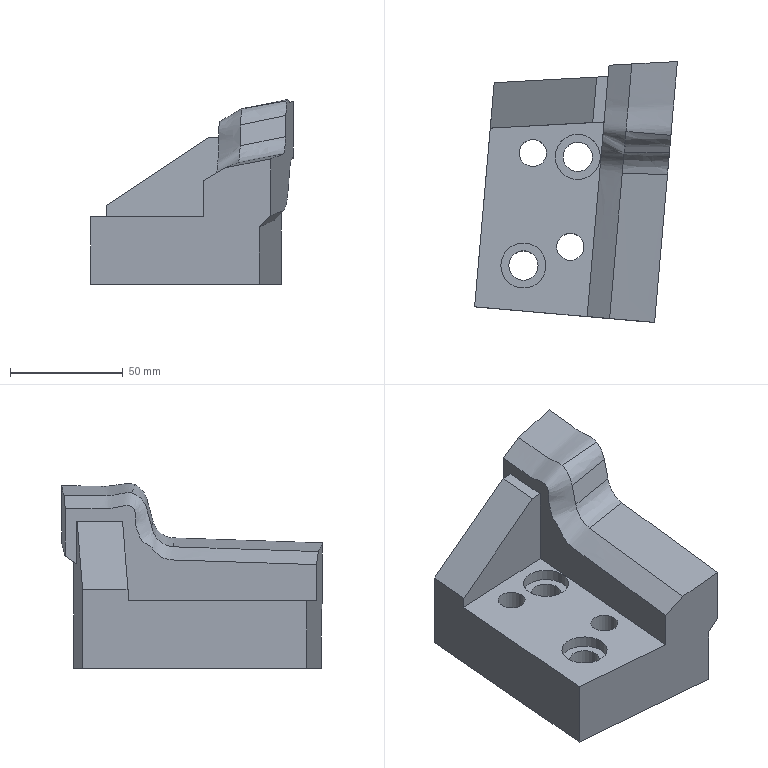Part | NX | features solid 2 | 1 solid | 28 faces | box 89.8 x 115.496 x 81.88 mm | volume 343642 mm3 | plane 11 | spline 11 | cylinder 6 | commonest cylinder face diameters 12 x2 13 x2 20 x2